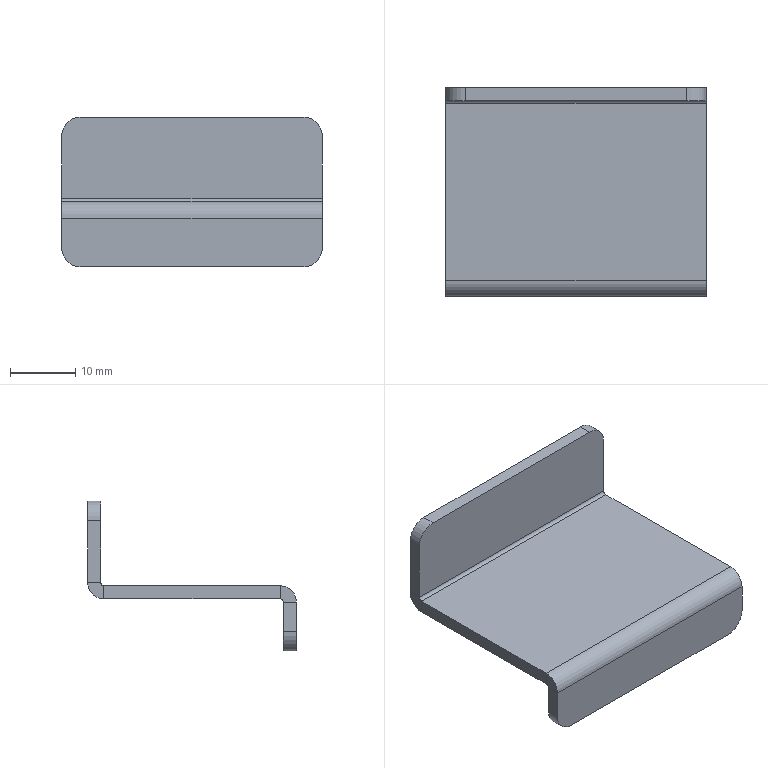Part | SolidWorks | features BaseBody 1 | 1 solid | 26 faces | box 40 x 32 x 23 mm | volume 4122 mm3 | plane 18 | cylinder 8 | commonest cylinder face diameters 6 x4 1 x2 5 x2
STEP:
#1=CARTESIAN_POINT('',(17.,-16.,-10.));
#2=VERTEX_POINT('',#1);
#3=CARTESIAN_POINT('',(20.,-16.,-7.));
#4=VERTEX_POINT('',#3);
#5=CARTESIAN_POINT('',(17.,-16.,-7.));
#6=DIRECTION('',(0.,-1.,0.));
#7=DIRECTION('',(0.,0.,-1.));
#8=AXIS2_PLACEMENT_3D('',#5,#6,#7);
#9=CIRCLE('',#8,3.);
#10=EDGE_CURVE('',#2,#4,#9,.T.);
#11=ORIENTED_EDGE('',*,*,#10,.F.);
#12=CARTESIAN_POINT('',(17.,-14.,-10.));
#13=VERTEX_POINT('',#12);
#14=CARTESIAN_POINT('',(17.,-16.,-10.));
#15=DIRECTION('',(0.,-1.,0.));
#16=VECTOR('',#15,1000.);
#17=LINE('',#14,#16);
#18=EDGE_CURVE('',#13,#2,#17,.T.);
#19=ORIENTED_EDGE('',*,*,#18,.F.);
#20=CARTESIAN_POINT('',(20.,-14.,-7.));
#21=VERTEX_POINT('',#20);
#22=CARTESIAN_POINT('',(17.,-14.,-7.));
#23=DIRECTION('',(0.,1.,0.));
#24=DIRECTION('',(0.,0.,-1.));
#25=AXIS2_PLACEMENT_3D('',#22,#23,#24);
#26=CIRCLE('',#25,3.);
#27=EDGE_CURVE('',#21,#13,#26,.T.);
#28=ORIENTED_EDGE('',*,*,#27,.F.);
#29=CARTESIAN_POINT('',(20.,-16.,-7.));
#30=DIRECTION('',(0.,1.,0.));
#31=VECTOR('',#30,1000.);
#32=LINE('',#29,#31);
#33=EDGE_CURVE('',#4,#21,#32,.T.);
#34=ORIENTED_EDGE('',*,*,#33,.F.);
#35=EDGE_LOOP('',(#11,#19,#28,#34));
#36=FACE_OUTER_BOUND('',#35,.T.);
#37=CARTESIAN_POINT('',(17.,-16.,-7.));
#38=DIRECTION('',(0.,1.,0.));
#39=DIRECTION('',(0.,0.,1.));
#40=AXIS2_PLACEMENT_3D('',#37,#38,#39);
#41=CYLINDRICAL_SURFACE('',#40,3.);
#42=ADVANCED_FACE('',(#36),#41,.T.);
#43=CARTESIAN_POINT('',(-20.,-16.,-7.));
#44=VERTEX_POINT('',#43);
#45=CARTESIAN_POINT('',(-17.,-16.,-10.));
#46=VERTEX_POINT('',#45);
#47=CARTESIAN_POINT('',(-17.,-16.,-7.));
#48=DIRECTION('',(0.,-1.,0.));
#49=DIRECTION('',(0.,0.,-1.));
#50=AXIS2_PLACEMENT_3D('',#47,#48,#49);
#51=CIRCLE('',#50,3.);
#52=EDGE_CURVE('',#44,#46,#51,.T.);
#53=ORIENTED_EDGE('',*,*,#52,.F.);
#54=CARTESIAN_POINT('',(-20.,-14.,-7.));
#55=VERTEX_POINT('',#54);
#56=CARTESIAN_POINT('',(-20.,-16.,-7.));
#57=DIRECTION('',(0.,-1.,0.));
#58=VECTOR('',#57,1000.);
#59=LINE('',#56,#58);
#60=EDGE_CURVE('',#55,#44,#59,.T.);
#61=ORIENTED_EDGE('',*,*,#60,.F.);
#62=CARTESIAN_POINT('',(-17.,-14.,-10.));
#63=VERTEX_POINT('',#62);
#64=CARTESIAN_POINT('',(-17.,-14.,-7.));
#65=DIRECTION('',(0.,1.,0.));
#66=DIRECTION('',(0.,0.,-1.));
#67=AXIS2_PLACEMENT_3D('',#64,#65,#66);
#68=CIRCLE('',#67,3.);
#69=EDGE_CURVE('',#63,#55,#68,.T.);
#70=ORIENTED_EDGE('',*,*,#69,.F.);
#71=CARTESIAN_POINT('',(-17.,-16.,-10.));
#72=DIRECTION('',(0.,1.,0.));
#73=VECTOR('',#72,1000.);
#74=LINE('',#71,#73);
#75=EDGE_CURVE('',#46,#63,#74,.T.);
#76=ORIENTED_EDGE('',*,*,#75,.F.);
#77=EDGE_LOOP('',(#53,#61,#70,#76));
#78=FACE_OUTER_BOUND('',#77,.T.);
#79=CARTESIAN_POINT('',(-17.,-16.,-7.));
#80=DIRECTION('',(0.,1.,0.));
#81=DIRECTION('',(0.,0.,1.));
#82=AXIS2_PLACEMENT_3D('',#79,#80,#81);
#83=CYLINDRICAL_SURFACE('',#82,3.);
#84=ADVANCED_FACE('',(#78),#83,.T.);
#85=CARTESIAN_POINT('',(17.,16.,13.));
#86=VERTEX_POINT('',#85);
#87=CARTESIAN_POINT('',(20.,16.,10.));
#88=VERTEX_POINT('',#87);
#89=CARTESIAN_POINT('',(17.,16.,10.));
#90=DIRECTION('',(0.,1.,0.));
#91=DIRECTION('',(0.,0.,-1.));
#92=AXIS2_PLACEMENT_3D('',#89,#90,#91);
#93=CIRCLE('',#92,3.);
#94=EDGE_CURVE('',#86,#88,#93,.T.);
#95=ORIENTED_EDGE('',*,*,#94,.F.);
#96=CARTESIAN_POINT('',(17.,14.,13.));
#97=VERTEX_POINT('',#96);
#98=CARTESIAN_POINT('',(17.,16.,13.));
#99=DIRECTION('',(0.,1.,0.));
#100=VECTOR('',#99,1000.);
#101=LINE('',#98,#100);
#102=EDGE_CURVE('',#97,#86,#101,.T.);
#103=ORIENTED_EDGE('',*,*,#102,.F.);
#104=CARTESIAN_POINT('',(20.,14.,10.));
#105=VERTEX_POINT('',#104);
#106=CARTESIAN_POINT('',(17.,14.,10.));
#107=DIRECTION('',(0.,-1.,0.));
#108=DIRECTION('',(0.,0.,-1.));
#109=AXIS2_PLACEMENT_3D('',#106,#107,#108);
#110=CIRCLE('',#109,3.);
#111=EDGE_CURVE('',#105,#97,#110,.T.);
#112=ORIENTED_EDGE('',*,*,#111,.F.);
#113=CARTESIAN_POINT('',(20.,16.,10.));
#114=DIRECTION('',(0.,-1.,0.));
#115=VECTOR('',#114,1000.);
#116=LINE('',#113,#115);
#117=EDGE_CURVE('',#88,#105,#116,.T.);
#118=ORIENTED_EDGE('',*,*,#117,.F.);
#119=EDGE_LOOP('',(#95,#103,#112,#118));
#120=FACE_OUTER_BOUND('',#119,.T.);
#121=CARTESIAN_POINT('',(17.,16.,10.));
#122=DIRECTION('',(0.,-1.,0.));
#123=DIRECTION('',(0.,0.,-1.));
#124=AXIS2_PLACEMENT_3D('',#121,#122,#123);
#125=CYLINDRICAL_SURFACE('',#124,3.);
#126=ADVANCED_FACE('',(#120),#125,.T.);
#127=CARTESIAN_POINT('',(-20.,16.,10.));
#128=VERTEX_POINT('',#127);
#129=CARTESIAN_POINT('',(-17.,16.,13.));
#130=VERTEX_POINT('',#129);
#131=CARTESIAN_POINT('',(-17.,16.,10.));
#132=DIRECTION('',(0.,1.,0.));
#133=DIRECTION('',(0.,0.,-1.));
#134=AXIS2_PLACEMENT_3D('',#131,#132,#133);
#135=CIRCLE('',#134,3.);
#136=EDGE_CURVE('',#128,#130,#135,.T.);
#137=ORIENTED_EDGE('',*,*,#136,.F.);
#138=CARTESIAN_POINT('',(-20.,14.,10.));
#139=VERTEX_POINT('',#138);
#140=CARTESIAN_POINT('',(-20.,16.,10.));
#141=DIRECTION('',(0.,1.,0.));
#142=VECTOR('',#141,1000.);
#143=LINE('',#140,#142);
#144=EDGE_CURVE('',#139,#128,#143,.T.);
#145=ORIENTED_EDGE('',*,*,#144,.F.);
#146=CARTESIAN_POINT('',(-17.,14.,13.));
#147=VERTEX_POINT('',#146);
#148=CARTESIAN_POINT('',(-17.,14.,10.));
#149=DIRECTION('',(0.,-1.,0.));
#150=DIRECTION('',(0.,0.,-1.));
#151=AXIS2_PLACEMENT_3D('',#148,#149,#150);
#152=CIRCLE('',#151,3.);
#153=EDGE_CURVE('',#147,#139,#152,.T.);
#154=ORIENTED_EDGE('',*,*,#153,.F.);
#155=CARTESIAN_POINT('',(-17.,16.,13.));
#156=DIRECTION('',(0.,-1.,0.));
#157=VECTOR('',#156,1000.);
#158=LINE('',#155,#157);
#159=EDGE_CURVE('',#130,#147,#158,.T.);
#160=ORIENTED_EDGE('',*,*,#159,.F.);
#161=EDGE_LOOP('',(#137,#145,#154,#160));
#162=FACE_OUTER_BOUND('',#161,.T.);
#163=CARTESIAN_POINT('',(-17.,16.,10.));
#164=DIRECTION('',(0.,-1.,0.));
#165=DIRECTION('',(0.,0.,-1.));
#166=AXIS2_PLACEMENT_3D('',#163,#164,#165);
#167=CYLINDRICAL_SURFACE('',#166,3.);
#168=ADVANCED_FACE('',(#162),#167,.T.);
#169=CARTESIAN_POINT('',(0.,16.,13.));
#170=DIRECTION('',(1.,0.,0.));
#171=VECTOR('',#170,1000.);
#172=LINE('',#169,#171);
#173=EDGE_CURVE('',#130,#86,#172,.T.);
#174=ORIENTED_EDGE('',*,*,#173,.F.);
#175=ORIENTED_EDGE('',*,*,#159,.T.);
#176=CARTESIAN_POINT('',(20.,14.,13.));
#177=DIRECTION('',(1.,0.,0.));
#178=VECTOR('',#177,1000.);
#179=LINE('',#176,#178);
#180=EDGE_CURVE('',#147,#97,#179,.T.);
#181=ORIENTED_EDGE('',*,*,#180,.T.);
#182=ORIENTED_EDGE('',*,*,#102,.T.);
#183=EDGE_LOOP('',(#174,#175,#181,#182));
#184=FACE_OUTER_BOUND('',#183,.T.);
#185=CARTESIAN_POINT('',(20.,16.,13.));
#186=DIRECTION('',(0.,0.,-1.));
#187=DIRECTION('',(0.,-1.,0.));
#188=AXIS2_PLACEMENT_3D('',#185,#186,#187);
#189=PLANE('',#188);
#190=ADVANCED_FACE('',(#184),#189,.F.);
#191=ORIENTED_EDGE('',*,*,#180,.F.);
#192=ORIENTED_EDGE('',*,*,#153,.T.);
#193=CARTESIAN_POINT('',(-20.,14.,0.5));
#194=VERTEX_POINT('',#193);
#195=CARTESIAN_POINT('',(-20.,14.,13.));
#196=DIRECTION('',(0.,0.,1.));
#197=VECTOR('',#196,1000.);
#198=LINE('',#195,#197);
#199=EDGE_CURVE('',#194,#139,#198,.T.);
#200=ORIENTED_EDGE('',*,*,#199,.F.);
#201=CARTESIAN_POINT('',(20.,14.,0.5));
#202=VERTEX_POINT('',#201);
#203=CARTESIAN_POINT('',(20.,14.,0.5));
#204=DIRECTION('',(-1.,0.,0.));
#205=VECTOR('',#204,1000.);
#206=LINE('',#203,#205);
#207=EDGE_CURVE('',#202,#194,#206,.T.);
#208=ORIENTED_EDGE('',*,*,#207,.F.);
#209=CARTESIAN_POINT('',(20.,14.,0.));
#210=DIRECTION('',(0.,0.,-1.));
#211=VECTOR('',#210,1000.);
#212=LINE('',#209,#211);
#213=EDGE_CURVE('',#105,#202,#212,.T.);
#214=ORIENTED_EDGE('',*,*,#213,.F.);
#215=ORIENTED_EDGE('',*,*,#111,.T.);
#216=EDGE_LOOP('',(#191,#192,#200,#208,#214,#215));
#217=FACE_OUTER_BOUND('',#216,.T.);
#218=CARTESIAN_POINT('',(0.,14.,0.));
#219=DIRECTION('',(0.,-1.,0.));
#220=DIRECTION('',(-1.,0.,0.));
#221=AXIS2_PLACEMENT_3D('',#218,#219,#220);
#222=PLANE('',#221);
#223=ADVANCED_FACE('',(#217),#222,.T.);
#224=CARTESIAN_POINT('',(-20.,16.,0.5));
#225=VERTEX_POINT('',#224);
#226=CARTESIAN_POINT('',(-20.,16.,0.));
#227=DIRECTION('',(0.,0.,1.));
#228=VECTOR('',#227,1000.);
#229=LINE('',#226,#228);
#230=EDGE_CURVE('',#225,#128,#229,.T.);
#231=ORIENTED_EDGE('',*,*,#230,.T.);
#232=ORIENTED_EDGE('',*,*,#136,.T.);
#233=ORIENTED_EDGE('',*,*,#173,.T.);
#234=ORIENTED_EDGE('',*,*,#94,.T.);
#235=CARTESIAN_POINT('',(20.,16.,0.5));
#236=VERTEX_POINT('',#235);
#237=CARTESIAN_POINT('',(20.,16.,0.));
#238=DIRECTION('',(0.,0.,-1.));
#239=VECTOR('',#238,1000.);
#240=LINE('',#237,#239);
#241=EDGE_CURVE('',#88,#236,#240,.T.);
#242=ORIENTED_EDGE('',*,*,#241,.T.);
#243=CARTESIAN_POINT('',(20.,16.,0.5));
#244=DIRECTION('',(1.,0.,0.));
#245=VECTOR('',#244,1000.);
#246=LINE('',#243,#245);
#247=EDGE_CURVE('',#225,#236,#246,.T.);
#248=ORIENTED_EDGE('',*,*,#247,.F.);
#249=EDGE_LOOP('',(#231,#232,#233,#234,#242,#248));
#250=FACE_OUTER_BOUND('',#249,.T.);
#251=CARTESIAN_POINT('',(0.,16.,0.));
#252=DIRECTION('',(0.,-1.,0.));
#253=DIRECTION('',(-1.,0.,0.));
#254=AXIS2_PLACEMENT_3D('',#251,#252,#253);
#255=PLANE('',#254);
#256=ADVANCED_FACE('',(#250),#255,.F.);
#257=ORIENTED_EDGE('',*,*,#199,.T.);
#258=ORIENTED_EDGE('',*,*,#144,.T.);
#259=ORIENTED_EDGE('',*,*,#230,.F.);
#260=CARTESIAN_POINT('',(-20.,14.,0.5));
#261=DIRECTION('',(0.,1.,0.));
#262=VECTOR('',#261,1000.);
#263=LINE('',#260,#262);
#264=EDGE_CURVE('',#194,#225,#263,.T.);
#265=ORIENTED_EDGE('',*,*,#264,.F.);
#266=EDGE_LOOP('',(#257,#258,#259,#265));
#267=FACE_OUTER_BOUND('',#266,.T.);
#268=CARTESIAN_POINT('',(-20.,16.,13.));
#269=DIRECTION('',(1.,0.,0.));
#270=DIRECTION('',(0.,1.,0.));
#271=AXIS2_PLACEMENT_3D('',#268,#269,#270);
#272=PLANE('',#271);
#273=ADVANCED_FACE('',(#267),#272,.F.);
#274=ORIENTED_EDGE('',*,*,#241,.F.);
#275=ORIENTED_EDGE('',*,*,#117,.T.);
#276=ORIENTED_EDGE('',*,*,#213,.T.);
#277=CARTESIAN_POINT('',(20.,16.,0.5));
#278=DIRECTION('',(0.,1.,0.));
#279=VECTOR('',#278,1000.);
#280=LINE('',#277,#279);
#281=EDGE_CURVE('',#202,#236,#280,.T.);
#282=ORIENTED_EDGE('',*,*,#281,.T.);
#283=EDGE_LOOP('',(#274,#275,#276,#282));
#284=FACE_OUTER_BOUND('',#283,.T.);
#285=CARTESIAN_POINT('',(20.,16.,0.));
#286=DIRECTION('',(-1.,0.,0.));
#287=DIRECTION('',(0.,0.,1.));
#288=AXIS2_PLACEMENT_3D('',#285,#286,#287);
#289=PLANE('',#288);
#290=ADVANCED_FACE('',(#284),#289,.F.);
#291=CARTESIAN_POINT('',(-20.,13.5,0.));
#292=VERTEX_POINT('',#291);
#293=CARTESIAN_POINT('',(20.,13.5,0.));
#294=VERTEX_POINT('',#293);
#295=CARTESIAN_POINT('',(-20.,13.5,0.));
#296=DIRECTION('',(1.,0.,0.));
#297=VECTOR('',#296,1000.);
#298=LINE('',#295,#297);
#299=EDGE_CURVE('',#292,#294,#298,.T.);
#300=ORIENTED_EDGE('',*,*,#299,.T.);
#301=CARTESIAN_POINT('',(20.,13.5,0.5));
#302=DIRECTION('',(1.,0.,0.));
#303=DIRECTION('',(0.,0.,1.));
#304=AXIS2_PLACEMENT_3D('',#301,#302,#303);
#305=CIRCLE('',#304,0.5);
#306=EDGE_CURVE('',#294,#202,#305,.T.);
#307=ORIENTED_EDGE('',*,*,#306,.T.);
#308=ORIENTED_EDGE('',*,*,#207,.T.);
#309=CARTESIAN_POINT('',(-20.,13.5,0.5));
#310=DIRECTION('',(-1.,0.,0.));
#311=DIRECTION('',(0.,0.,1.));
#312=AXIS2_PLACEMENT_3D('',#309,#310,#311);
#313=CIRCLE('',#312,0.5);
#314=EDGE_CURVE('',#194,#292,#313,.T.);
#315=ORIENTED_EDGE('',*,*,#314,.T.);
#316=EDGE_LOOP('',(#300,#307,#308,#315));
#317=FACE_OUTER_BOUND('',#316,.T.);
#318=CARTESIAN_POINT('',(-20.,13.5,0.5));
#319=DIRECTION('',(-1.,0.,0.));
#320=DIRECTION('',(0.,1.,0.));
#321=AXIS2_PLACEMENT_3D('',#318,#319,#320);
#322=CYLINDRICAL_SURFACE('',#321,0.5);
#323=ADVANCED_FACE('',(#317),#322,.F.);
#324=CARTESIAN_POINT('',(-20.,13.5,-2.));
#325=VERTEX_POINT('',#324);
#326=CARTESIAN_POINT('',(20.,13.5,-2.));
#327=VERTEX_POINT('',#326);
#328=CARTESIAN_POINT('',(-20.,13.5,-2.));
#329=DIRECTION('',(1.,0.,0.));
#330=VECTOR('',#329,1000.);
#331=LINE('',#328,#330);
#332=EDGE_CURVE('',#325,#327,#331,.T.);
#333=ORIENTED_EDGE('',*,*,#332,.F.);
#334=CARTESIAN_POINT('',(-20.,13.5,0.5));
#335=DIRECTION('',(-1.,0.,0.));
#336=DIRECTION('',(0.,0.,1.));
#337=AXIS2_PLACEMENT_3D('',#334,#335,#336);
#338=CIRCLE('',#337,2.5);
#339=EDGE_CURVE('',#225,#325,#338,.T.);
#340=ORIENTED_EDGE('',*,*,#339,.F.);
#341=ORIENTED_EDGE('',*,*,#247,.T.);
#342=CARTESIAN_POINT('',(20.,13.5,0.5));
#343=DIRECTION('',(1.,0.,0.));
#344=DIRECTION('',(0.,0.,1.));
#345=AXIS2_PLACEMENT_3D('',#342,#343,#344);
#346=CIRCLE('',#345,2.5);
#347=EDGE_CURVE('',#327,#236,#346,.T.);
#348=ORIENTED_EDGE('',*,*,#347,.F.);
#349=EDGE_LOOP('',(#333,#340,#341,#348));
#350=FACE_OUTER_BOUND('',#349,.T.);
#351=CARTESIAN_POINT('',(-20.,13.5,0.5));
#352=DIRECTION('',(-1.,0.,0.));
#353=DIRECTION('',(0.,1.,0.));
#354=AXIS2_PLACEMENT_3D('',#351,#352,#353);
#355=CYLINDRICAL_SURFACE('',#354,2.5);
#356=ADVANCED_FACE('',(#350),#355,.T.);
#357=ORIENTED_EDGE('',*,*,#314,.F.);
#358=ORIENTED_EDGE('',*,*,#264,.T.);
#359=ORIENTED_EDGE('',*,*,#339,.T.);
#360=CARTESIAN_POINT('',(-20.,13.5,0.));
#361=DIRECTION('',(0.,0.,-1.));
#362=VECTOR('',#361,1000.);
#363=LINE('',#360,#362);
#364=EDGE_CURVE('',#292,#325,#363,.T.);
#365=ORIENTED_EDGE('',*,*,#364,.F.);
#366=EDGE_LOOP('',(#357,#358,#359,#365));
#367=FACE_OUTER_BOUND('',#366,.T.);
#368=CARTESIAN_POINT('',(-20.,13.5,0.5));
#369=DIRECTION('',(1.,0.,0.));
#370=DIRECTION('',(0.,1.,0.));
#371=AXIS2_PLACEMENT_3D('',#368,#369,#370);
#372=PLANE('',#371);
#373=ADVANCED_FACE('',(#367),#372,.F.);
#374=ORIENTED_EDGE('',*,*,#281,.F.);
#375=ORIENTED_EDGE('',*,*,#306,.F.);
#376=CARTESIAN_POINT('',(20.,13.5,0.));
#377=DIRECTION('',(0.,0.,-1.));
#378=VECTOR('',#377,1000.);
#379=LINE('',#376,#378);
#380=EDGE_CURVE('',#294,#327,#379,.T.);
#381=ORIENTED_EDGE('',*,*,#380,.T.);
#382=ORIENTED_EDGE('',*,*,#347,.T.);
#383=EDGE_LOOP('',(#374,#375,#381,#382));
#384=FACE_OUTER_BOUND('',#383,.T.);
#385=CARTESIAN_POINT('',(20.,13.5,0.5));
#386=DIRECTION('',(1.,0.,0.));
#387=DIRECTION('',(0.,1.,0.));
#388=AXIS2_PLACEMENT_3D('',#385,#386,#387);
#389=PLANE('',#388);
#390=ADVANCED_FACE('',(#384),#389,.T.);
#391=CARTESIAN_POINT('',(-20.,-16.,-10.));
#392=DIRECTION('',(-1.,0.,0.));
#393=VECTOR('',#392,1000.);
#394=LINE('',#391,#393);
#395=EDGE_CURVE('',#2,#46,#394,.T.);
#396=ORIENTED_EDGE('',*,*,#395,.T.);
#397=ORIENTED_EDGE('',*,*,#75,.T.);
#398=CARTESIAN_POINT('',(0.,-14.,-10.));
#399=DIRECTION('',(-1.,0.,0.));
#400=VECTOR('',#399,1000.);
#401=LINE('',#398,#400);
#402=EDGE_CURVE('',#13,#63,#401,.T.);
#403=ORIENTED_EDGE('',*,*,#402,.F.);
#404=ORIENTED_EDGE('',*,*,#18,.T.);
#405=EDGE_LOOP('',(#396,#397,#403,#404));
#406=FACE_OUTER_BOUND('',#405,.T.);
#407=CARTESIAN_POINT('',(-20.,-16.,-10.));
#408=DIRECTION('',(0.,0.,-1.));
#409=DIRECTION('',(0.,-1.,0.));
#410=AXIS2_PLACEMENT_3D('',#407,#408,#409);
#411=PLANE('',#410);
#412=ADVANCED_FACE('',(#406),#411,.T.);
#413=ORIENTED_EDGE('',*,*,#402,.T.);
#414=ORIENTED_EDGE('',*,*,#69,.T.);
#415=CARTESIAN_POINT('',(-20.,-14.,-2.5));
#416=VERTEX_POINT('',#415);
#417=CARTESIAN_POINT('',(-20.,-14.,0.));
#418=DIRECTION('',(0.,0.,1.));
#419=VECTOR('',#418,1000.);
#420=LINE('',#417,#419);
#421=EDGE_CURVE('',#55,#416,#420,.T.);
#422=ORIENTED_EDGE('',*,*,#421,.T.);
#423=CARTESIAN_POINT('',(20.,-14.,-2.5));
#424=VERTEX_POINT('',#423);
#425=CARTESIAN_POINT('',(20.,-14.,-2.5));
#426=DIRECTION('',(-1.,0.,0.));
#427=VECTOR('',#426,1000.);
#428=LINE('',#425,#427);
#429=EDGE_CURVE('',#424,#416,#428,.T.);
#430=ORIENTED_EDGE('',*,*,#429,.F.);
#431=CARTESIAN_POINT('',(20.,-14.,0.));
#432=DIRECTION('',(0.,0.,-1.));
#433=VECTOR('',#432,1000.);
#434=LINE('',#431,#433);
#435=EDGE_CURVE('',#424,#21,#434,.T.);
#436=ORIENTED_EDGE('',*,*,#435,.T.);
#437=ORIENTED_EDGE('',*,*,#27,.T.);
#438=EDGE_LOOP('',(#413,#414,#422,#430,#436,#437));
#439=FACE_OUTER_BOUND('',#438,.T.);
#440=CARTESIAN_POINT('',(0.,-14.,0.));
#441=DIRECTION('',(0.,-1.,0.));
#442=DIRECTION('',(-1.,0.,0.));
#443=AXIS2_PLACEMENT_3D('',#440,#441,#442);
#444=PLANE('',#443);
#445=ADVANCED_FACE('',(#439),#444,.F.);
#446=CARTESIAN_POINT('',(-20.,-16.,-2.5));
#447=VERTEX_POINT('',#446);
#448=CARTESIAN_POINT('',(-20.,-16.,-2.));
#449=DIRECTION('',(0.,0.,1.));
#450=VECTOR('',#449,1000.);
#451=LINE('',#448,#450);
#452=EDGE_CURVE('',#44,#447,#451,.T.);
#453=ORIENTED_EDGE('',*,*,#452,.F.);
#454=ORIENTED_EDGE('',*,*,#52,.T.);
#455=ORIENTED_EDGE('',*,*,#395,.F.);
#456=ORIENTED_EDGE('',*,*,#10,.T.);
#457=CARTESIAN_POINT('',(20.,-16.,-2.5));
#458=VERTEX_POINT('',#457);
#459=CARTESIAN_POINT('',(20.,-16.,-10.));
#460=DIRECTION('',(0.,0.,-1.));
#461=VECTOR('',#460,1000.);
#462=LINE('',#459,#461);
#463=EDGE_CURVE('',#458,#4,#462,.T.);
#464=ORIENTED_EDGE('',*,*,#463,.F.);
#465=CARTESIAN_POINT('',(0.,-16.,-2.5));
#466=DIRECTION('',(-1.,0.,0.));
#467=VECTOR('',#466,1000.);
#468=LINE('',#465,#467);
#469=EDGE_CURVE('',#458,#447,#468,.T.);
#470=ORIENTED_EDGE('',*,*,#469,.T.);
#471=EDGE_LOOP('',(#453,#454,#455,#456,#464,#470));
#472=FACE_OUTER_BOUND('',#471,.T.);
#473=CARTESIAN_POINT('',(0.,-16.,0.));
#474=DIRECTION('',(0.,-1.,0.));
#475=DIRECTION('',(-1.,0.,0.));
#476=AXIS2_PLACEMENT_3D('',#473,#474,#475);
#477=PLANE('',#476);
#478=ADVANCED_FACE('',(#472),#477,.T.);
#479=ORIENTED_EDGE('',*,*,#463,.T.);
#480=ORIENTED_EDGE('',*,*,#33,.T.);
#481=ORIENTED_EDGE('',*,*,#435,.F.);
#482=CARTESIAN_POINT('',(20.,-16.,-2.5));
#483=DIRECTION('',(0.,-1.,0.));
#484=VECTOR('',#483,1000.);
#485=LINE('',#482,#484);
#486=EDGE_CURVE('',#424,#458,#485,.T.);
#487=ORIENTED_EDGE('',*,*,#486,.T.);
#488=EDGE_LOOP('',(#479,#480,#481,#487));
#489=FACE_OUTER_BOUND('',#488,.T.);
#490=CARTESIAN_POINT('',(20.,-16.,-10.));
#491=DIRECTION('',(1.,0.,0.));
#492=DIRECTION('',(0.,0.,1.));
#493=AXIS2_PLACEMENT_3D('',#490,#491,#492);
#494=PLANE('',#493);
#495=ADVANCED_FACE('',(#489),#494,.T.);
#496=ORIENTED_EDGE('',*,*,#421,.F.);
#497=ORIENTED_EDGE('',*,*,#60,.T.);
#498=ORIENTED_EDGE('',*,*,#452,.T.);
#499=CARTESIAN_POINT('',(-20.,-14.,-2.5));
#500=DIRECTION('',(0.,-1.,0.));
#501=VECTOR('',#500,1000.);
#502=LINE('',#499,#501);
#503=EDGE_CURVE('',#416,#447,#502,.T.);
#504=ORIENTED_EDGE('',*,*,#503,.F.);
#505=EDGE_LOOP('',(#496,#497,#498,#504));
#506=FACE_OUTER_BOUND('',#505,.T.);
#507=CARTESIAN_POINT('',(-20.,-16.,-2.));
#508=DIRECTION('',(-1.,0.,0.));
#509=DIRECTION('',(0.,0.,1.));
#510=AXIS2_PLACEMENT_3D('',#507,#508,#509);
#511=PLANE('',#510);
#512=ADVANCED_FACE('',(#506),#511,.T.);
#513=CARTESIAN_POINT('',(-20.,-13.5,-2.));
#514=VERTEX_POINT('',#513);
#515=CARTESIAN_POINT('',(20.,-13.5,-2.));
#516=VERTEX_POINT('',#515);
#517=CARTESIAN_POINT('',(-20.,-13.5,-2.));
#518=DIRECTION('',(1.,0.,0.));
#519=VECTOR('',#518,1000.);
#520=LINE('',#517,#519);
#521=EDGE_CURVE('',#514,#516,#520,.T.);
#522=ORIENTED_EDGE('',*,*,#521,.T.);
#523=CARTESIAN_POINT('',(20.,-13.5,-2.5));
#524=DIRECTION('',(1.,0.,0.));
#525=DIRECTION('',(0.,0.,1.));
#526=AXIS2_PLACEMENT_3D('',#523,#524,#525);
#527=CIRCLE('',#526,0.5);
#528=EDGE_CURVE('',#516,#424,#527,.T.);
#529=ORIENTED_EDGE('',*,*,#528,.T.);
#530=ORIENTED_EDGE('',*,*,#429,.T.);
#531=CARTESIAN_POINT('',(-20.,-13.5,-2.5));
#532=DIRECTION('',(-1.,0.,0.));
#533=DIRECTION('',(0.,0.,1.));
#534=AXIS2_PLACEMENT_3D('',#531,#532,#533);
#535=CIRCLE('',#534,0.5);
#536=EDGE_CURVE('',#416,#514,#535,.T.);
#537=ORIENTED_EDGE('',*,*,#536,.T.);
#538=EDGE_LOOP('',(#522,#529,#530,#537));
#539=FACE_OUTER_BOUND('',#538,.T.);
#540=CARTESIAN_POINT('',(-20.,-13.5,-2.5));
#541=DIRECTION('',(-1.,0.,0.));
#542=DIRECTION('',(0.,-1.,0.));
#543=AXIS2_PLACEMENT_3D('',#540,#541,#542);
#544=CYLINDRICAL_SURFACE('',#543,0.5);
#545=ADVANCED_FACE('',(#539),#544,.F.);
#546=CARTESIAN_POINT('',(-20.,-13.5,0.));
#547=VERTEX_POINT('',#546);
#548=CARTESIAN_POINT('',(20.,-13.5,0.));
#549=VERTEX_POINT('',#548);
#550=CARTESIAN_POINT('',(-20.,-13.5,0.));
#551=DIRECTION('',(1.,0.,0.));
#552=VECTOR('',#551,1000.);
#553=LINE('',#550,#552);
#554=EDGE_CURVE('',#547,#549,#553,.T.);
#555=ORIENTED_EDGE('',*,*,#554,.F.);
#556=CARTESIAN_POINT('',(-20.,-13.5,-2.5));
#557=DIRECTION('',(-1.,0.,0.));
#558=DIRECTION('',(0.,0.,1.));
#559=AXIS2_PLACEMENT_3D('',#556,#557,#558);
#560=CIRCLE('',#559,2.5);
#561=EDGE_CURVE('',#447,#547,#560,.T.);
#562=ORIENTED_EDGE('',*,*,#561,.F.);
#563=ORIENTED_EDGE('',*,*,#469,.F.);
#564=CARTESIAN_POINT('',(20.,-13.5,-2.5));
#565=DIRECTION('',(1.,0.,0.));
#566=DIRECTION('',(0.,0.,1.));
#567=AXIS2_PLACEMENT_3D('',#564,#565,#566);
#568=CIRCLE('',#567,2.5);
#569=EDGE_CURVE('',#549,#458,#568,.T.);
#570=ORIENTED_EDGE('',*,*,#569,.F.);
#571=EDGE_LOOP('',(#555,#562,#563,#570));
#572=FACE_OUTER_BOUND('',#571,.T.);
#573=CARTESIAN_POINT('',(-20.,-13.5,-2.5));
#574=DIRECTION('',(-1.,0.,0.));
#575=DIRECTION('',(0.,-1.,0.));
#576=AXIS2_PLACEMENT_3D('',#573,#574,#575);
#577=CYLINDRICAL_SURFACE('',#576,2.5);
#578=ADVANCED_FACE('',(#572),#577,.T.);
#579=ORIENTED_EDGE('',*,*,#536,.F.);
#580=ORIENTED_EDGE('',*,*,#503,.T.);
#581=ORIENTED_EDGE('',*,*,#561,.T.);
#582=CARTESIAN_POINT('',(-20.,-13.5,-2.));
#583=DIRECTION('',(0.,0.,1.));
#584=VECTOR('',#583,1000.);
#585=LINE('',#582,#584);
#586=EDGE_CURVE('',#514,#547,#585,.T.);
#587=ORIENTED_EDGE('',*,*,#586,.F.);
#588=EDGE_LOOP('',(#579,#580,#581,#587));
#589=FACE_OUTER_BOUND('',#588,.T.);
#590=CARTESIAN_POINT('',(-20.,-13.5,-2.5));
#591=DIRECTION('',(1.,0.,0.));
#592=DIRECTION('',(0.,1.,0.));
#593=AXIS2_PLACEMENT_3D('',#590,#591,#592);
#594=PLANE('',#593);
#595=ADVANCED_FACE('',(#589),#594,.F.);
#596=ORIENTED_EDGE('',*,*,#486,.F.);
#597=ORIENTED_EDGE('',*,*,#528,.F.);
#598=CARTESIAN_POINT('',(20.,-13.5,-2.));
#599=DIRECTION('',(0.,0.,1.));
#600=VECTOR('',#599,1000.);
#601=LINE('',#598,#600);
#602=EDGE_CURVE('',#516,#549,#601,.T.);
#603=ORIENTED_EDGE('',*,*,#602,.T.);
#604=ORIENTED_EDGE('',*,*,#569,.T.);
#605=EDGE_LOOP('',(#596,#597,#603,#604));
#606=FACE_OUTER_BOUND('',#605,.T.);
#607=CARTESIAN_POINT('',(20.,-13.5,-2.5));
#608=DIRECTION('',(1.,0.,0.));
#609=DIRECTION('',(0.,1.,0.));
#610=AXIS2_PLACEMENT_3D('',#607,#608,#609);
#611=PLANE('',#610);
#612=ADVANCED_FACE('',(#606),#611,.T.);
#613=ORIENTED_EDGE('',*,*,#380,.F.);
#614=CARTESIAN_POINT('',(20.,16.,0.));
#615=DIRECTION('',(0.,1.,0.));
#616=VECTOR('',#615,1000.);
#617=LINE('',#614,#616);
#618=EDGE_CURVE('',#549,#294,#617,.T.);
#619=ORIENTED_EDGE('',*,*,#618,.F.);
#620=ORIENTED_EDGE('',*,*,#602,.F.);
#621=CARTESIAN_POINT('',(20.,16.,-2.));
#622=DIRECTION('',(0.,1.,0.));
#623=VECTOR('',#622,1000.);
#624=LINE('',#621,#623);
#625=EDGE_CURVE('',#516,#327,#624,.T.);
#626=ORIENTED_EDGE('',*,*,#625,.T.);
#627=EDGE_LOOP('',(#613,#619,#620,#626));
#628=FACE_OUTER_BOUND('',#627,.T.);
#629=CARTESIAN_POINT('',(20.,16.,-2.));
#630=DIRECTION('',(1.,0.,0.));
#631=DIRECTION('',(0.,1.,0.));
#632=AXIS2_PLACEMENT_3D('',#629,#630,#631);
#633=PLANE('',#632);
#634=ADVANCED_FACE('',(#628),#633,.T.);
#635=ORIENTED_EDGE('',*,*,#618,.T.);
#636=ORIENTED_EDGE('',*,*,#299,.F.);
#637=CARTESIAN_POINT('',(-20.,16.,0.));
#638=DIRECTION('',(0.,-1.,0.));
#639=VECTOR('',#638,1000.);
#640=LINE('',#637,#639);
#641=EDGE_CURVE('',#292,#547,#640,.T.);
#642=ORIENTED_EDGE('',*,*,#641,.T.);
#643=ORIENTED_EDGE('',*,*,#554,.T.);
#644=EDGE_LOOP('',(#635,#636,#642,#643));
#645=FACE_OUTER_BOUND('',#644,.T.);
#646=CARTESIAN_POINT('',(0.,0.,0.));
#647=DIRECTION('',(0.,0.,1.));
#648=DIRECTION('',(1.,0.,0.));
#649=AXIS2_PLACEMENT_3D('',#646,#647,#648);
#650=PLANE('',#649);
#651=ADVANCED_FACE('',(#645),#650,.T.);
#652=ORIENTED_EDGE('',*,*,#332,.T.);
#653=ORIENTED_EDGE('',*,*,#625,.F.);
#654=ORIENTED_EDGE('',*,*,#521,.F.);
#655=CARTESIAN_POINT('',(-20.,16.,-2.));
#656=DIRECTION('',(0.,-1.,0.));
#657=VECTOR('',#656,1000.);
#658=LINE('',#655,#657);
#659=EDGE_CURVE('',#325,#514,#658,.T.);
#660=ORIENTED_EDGE('',*,*,#659,.F.);
#661=EDGE_LOOP('',(#652,#653,#654,#660));
#662=FACE_OUTER_BOUND('',#661,.T.);
#663=CARTESIAN_POINT('',(0.,0.,-2.));
#664=DIRECTION('',(0.,0.,1.));
#665=DIRECTION('',(1.,0.,0.));
#666=AXIS2_PLACEMENT_3D('',#663,#664,#665);
#667=PLANE('',#666);
#668=ADVANCED_FACE('',(#662),#667,.F.);
#669=ORIENTED_EDGE('',*,*,#641,.F.);
#670=ORIENTED_EDGE('',*,*,#364,.T.);
#671=ORIENTED_EDGE('',*,*,#659,.T.);
#672=ORIENTED_EDGE('',*,*,#586,.T.);
#673=EDGE_LOOP('',(#669,#670,#671,#672));
#674=FACE_OUTER_BOUND('',#673,.T.);
#675=CARTESIAN_POINT('',(-20.,16.,-2.));
#676=DIRECTION('',(-1.,0.,0.));
#677=DIRECTION('',(0.,1.,0.));
#678=AXIS2_PLACEMENT_3D('',#675,#676,#677);
#679=PLANE('',#678);
#680=ADVANCED_FACE('',(#674),#679,.T.);
#681=CLOSED_SHELL('',(#42,#84,#126,#168,#190,#223,#256,#273,#290,#323,#356,#373,#390,#412,#445,#478,#495,#512,#545,#578,#595,#612,#634,#651,#668,#680));
#682=MANIFOLD_SOLID_BREP('',#681);
#683=CARTESIAN_POINT('',(0.,0.,0.));
#684=DIRECTION('',(0.,0.,1.));
#685=DIRECTION('',(1.,0.,0.));
#686=AXIS2_PLACEMENT_3D('',#683,#684,#685);
#687=(LENGTH_UNIT()NAMED_UNIT(*)SI_UNIT(.MILLI.,.METRE.));
#688=UNCERTAINTY_MEASURE_WITH_UNIT(LENGTH_MEASURE(0.00001),#687,'','');
#689=(NAMED_UNIT(*)PLANE_ANGLE_UNIT()SI_UNIT($,.RADIAN.));
#690=(NAMED_UNIT(*)SI_UNIT($,.STERADIAN.)SOLID_ANGLE_UNIT());
#691=(GEOMETRIC_REPRESENTATION_CONTEXT(3)GLOBAL_UNCERTAINTY_ASSIGNED_CONTEXT((#688))GLOBAL_UNIT_ASSIGNED_CONTEXT((#687,#689,#690))REPRESENTATION_CONTEXT('',''));
#692=ADVANCED_BREP_SHAPE_REPRESENTATION('',(#682,#686),#691);